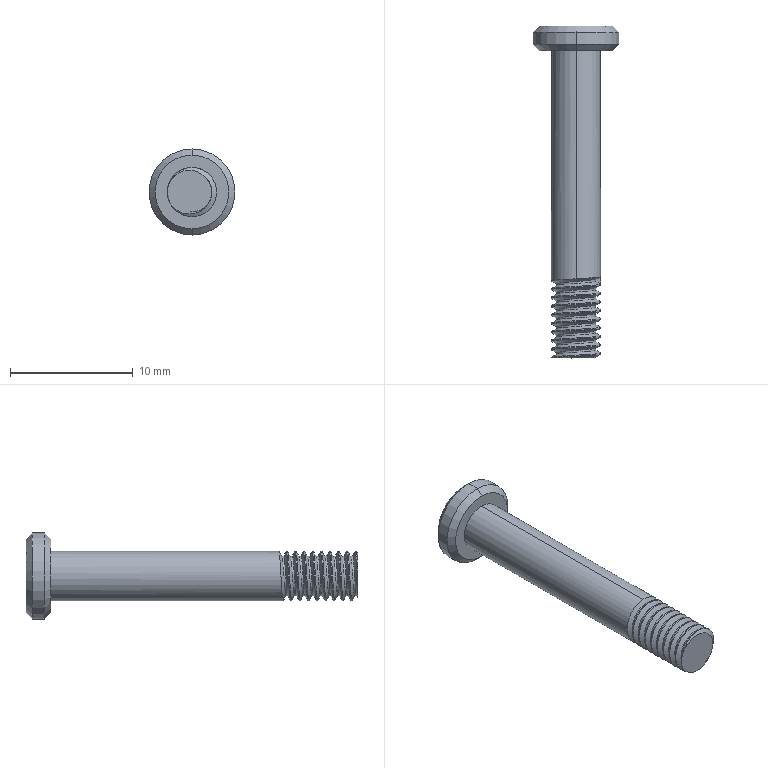Part | NX | features BREP 1 | 1 solid | 39 faces | box 7 x 27 x 7 mm | volume 340.818 mm3 | cylinder 22 | plane 11 | cone 4 | spline 2 | commonest cylinder face diameters 4 x19 7 x2 3.242 x1